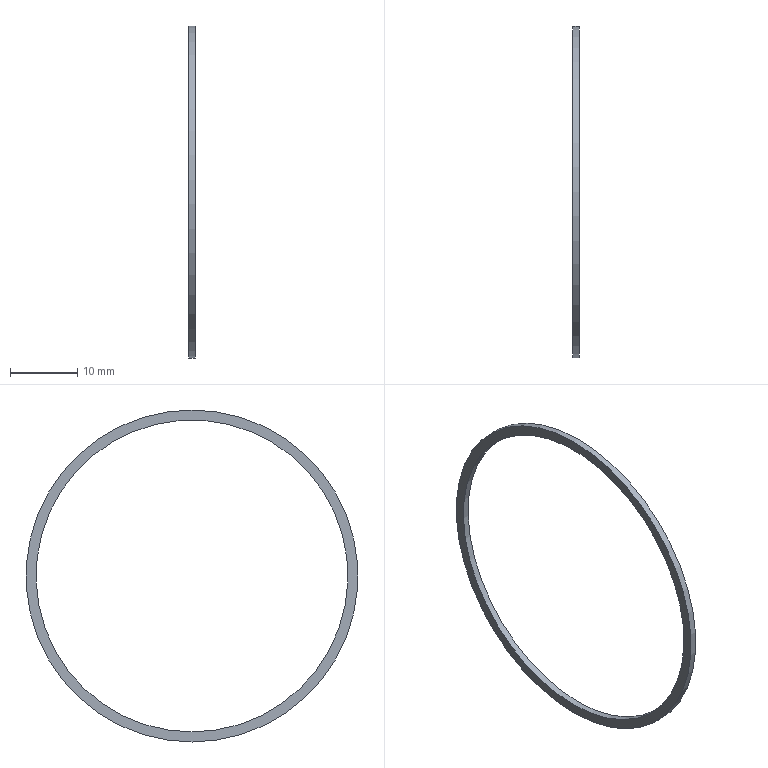Part | STEP file | Inner gasket of clamping device | 1 solid | 4 faces | box 1 x 49.5 x 49.5 mm | volume 226.195 mm3 | plane 2 | cylinder 2 | commonest cylinder face diameters 46.5 x1 49.5 x1
STEP:
#1=CARTESIAN_POINT('',(0.,0.,-24.75));
#2=VERTEX_POINT('',#1);
#3=CARTESIAN_POINT('',(0.,0.,0.));
#4=DIRECTION('',(1.,0.,0.));
#5=DIRECTION('',(0.,0.,-1.));
#6=AXIS2_PLACEMENT_3D('',#3,#4,#5);
#7=CIRCLE('',#6,24.75);
#8=EDGE_CURVE('',#2,#2,#7,.T.);
#9=ORIENTED_EDGE('',*,*,#8,.F.);
#10=EDGE_LOOP('',(#9));
#11=FACE_BOUND('',#10,.T.);
#12=CARTESIAN_POINT('',(0.,0.,-23.25));
#13=VERTEX_POINT('',#12);
#14=CARTESIAN_POINT('',(0.,0.,0.));
#15=DIRECTION('',(1.,0.,0.));
#16=DIRECTION('',(0.,0.,-1.));
#17=AXIS2_PLACEMENT_3D('',#14,#15,#16);
#18=CIRCLE('',#17,23.25);
#19=EDGE_CURVE('',#13,#13,#18,.T.);
#20=ORIENTED_EDGE('',*,*,#19,.T.);
#21=EDGE_LOOP('',(#20));
#22=FACE_BOUND('',#21,.T.);
#23=CARTESIAN_POINT('',(0.,0.,0.));
#24=DIRECTION('',(1.,0.,0.));
#25=DIRECTION('',(0.,0.,-1.));
#26=AXIS2_PLACEMENT_3D('',#23,#24,#25);
#27=PLANE('',#26);
#28=ADVANCED_FACE('',(#11,#22),#27,.F.);
#29=CARTESIAN_POINT('',(1.,0.,-24.75));
#30=VERTEX_POINT('',#29);
#31=CARTESIAN_POINT('',(1.,0.,0.));
#32=DIRECTION('',(1.,0.,0.));
#33=DIRECTION('',(0.,0.,-1.));
#34=AXIS2_PLACEMENT_3D('',#31,#32,#33);
#35=CIRCLE('',#34,24.75);
#36=EDGE_CURVE('',#30,#30,#35,.T.);
#37=ORIENTED_EDGE('',*,*,#36,.T.);
#38=EDGE_LOOP('',(#37));
#39=FACE_BOUND('',#38,.T.);
#40=CARTESIAN_POINT('',(1.,0.,-23.25));
#41=VERTEX_POINT('',#40);
#42=CARTESIAN_POINT('',(1.,0.,0.));
#43=DIRECTION('',(1.,0.,0.));
#44=DIRECTION('',(0.,0.,-1.));
#45=AXIS2_PLACEMENT_3D('',#42,#43,#44);
#46=CIRCLE('',#45,23.25);
#47=EDGE_CURVE('',#41,#41,#46,.F.);
#48=ORIENTED_EDGE('',*,*,#47,.T.);
#49=EDGE_LOOP('',(#48));
#50=FACE_BOUND('',#49,.T.);
#51=CARTESIAN_POINT('',(1.,0.,0.));
#52=DIRECTION('',(1.,0.,0.));
#53=DIRECTION('',(0.,0.,-1.));
#54=AXIS2_PLACEMENT_3D('',#51,#52,#53);
#55=PLANE('',#54);
#56=ADVANCED_FACE('',(#39,#50),#55,.T.);
#57=ORIENTED_EDGE('',*,*,#47,.F.);
#58=EDGE_LOOP('',(#57));
#59=FACE_OUTER_BOUND('',#58,.T.);
#60=ORIENTED_EDGE('',*,*,#19,.F.);
#61=EDGE_LOOP('',(#60));
#62=FACE_OUTER_BOUND('',#61,.T.);
#63=CARTESIAN_POINT('',(0.,0.,0.));
#64=DIRECTION('',(1.,0.,0.));
#65=DIRECTION('',(0.,0.,-1.));
#66=AXIS2_PLACEMENT_3D('',#63,#64,#65);
#67=CYLINDRICAL_SURFACE('',#66,23.25);
#68=ADVANCED_FACE('',(#59,#62),#67,.F.);
#69=ORIENTED_EDGE('',*,*,#36,.F.);
#70=EDGE_LOOP('',(#69));
#71=FACE_OUTER_BOUND('',#70,.T.);
#72=ORIENTED_EDGE('',*,*,#8,.T.);
#73=EDGE_LOOP('',(#72));
#74=FACE_OUTER_BOUND('',#73,.T.);
#75=CARTESIAN_POINT('',(0.,0.,0.));
#76=DIRECTION('',(1.,0.,0.));
#77=DIRECTION('',(0.,0.,-1.));
#78=AXIS2_PLACEMENT_3D('',#75,#76,#77);
#79=CYLINDRICAL_SURFACE('',#78,24.75);
#80=ADVANCED_FACE('',(#71,#74),#79,.T.);
#81=CLOSED_SHELL('',(#28,#56,#68,#80));
#82=MANIFOLD_SOLID_BREP('',#81);
#83=(LENGTH_UNIT()NAMED_UNIT(*)SI_UNIT(.MILLI.,.METRE.));
#84=UNCERTAINTY_MEASURE_WITH_UNIT(LENGTH_MEASURE(0.00001),#83,'','');
#85=(NAMED_UNIT(*)PLANE_ANGLE_UNIT()SI_UNIT($,.RADIAN.));
#86=(NAMED_UNIT(*)SI_UNIT($,.STERADIAN.)SOLID_ANGLE_UNIT());
#87=(GEOMETRIC_REPRESENTATION_CONTEXT(3)GLOBAL_UNCERTAINTY_ASSIGNED_CONTEXT((#84))GLOBAL_UNIT_ASSIGNED_CONTEXT((#83,#85,#86))REPRESENTATION_CONTEXT('',''));
#88=ADVANCED_BREP_SHAPE_REPRESENTATION('',(#82),#87);